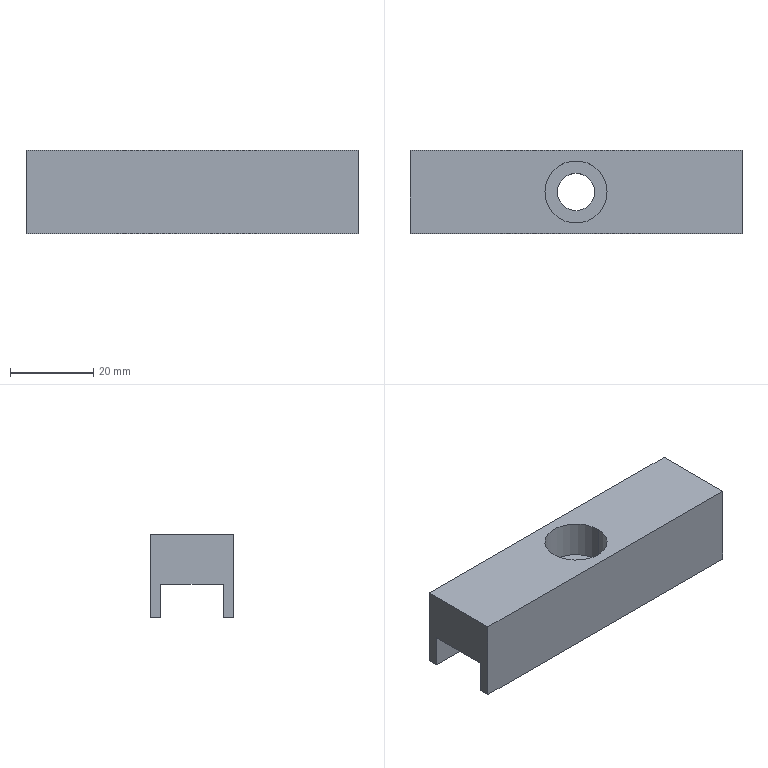Part | STEP file | Top plate part | 1 solid | 15 faces | box 80 x 20 x 20 mm | volume 20619 mm3 | plane 11 | cylinder 4 | commonest cylinder face diameters 9 x2 15 x2
STEP:
#1=CARTESIAN_POINT('',(0.,0.,0.));
#2=DIRECTION('',(0.,0.,1.));
#3=DIRECTION('',(1.,0.,0.));
#4=AXIS2_PLACEMENT_3D('',#1,#2,#3);
#5=CARTESIAN_POINT('',(7.5,0.,11.));
#6=VERTEX_POINT('',#5);
#7=CARTESIAN_POINT('',(7.5,0.,20.));
#8=VERTEX_POINT('',#7);
#9=CARTESIAN_POINT('',(7.5,0.,20.));
#10=DIRECTION('',(0.,0.,1.));
#11=VECTOR('',#10,1.);
#12=LINE('',#9,#11);
#13=CARTESIAN_POINT('',(0.,0.,20.));
#14=DIRECTION('',(0.,0.,1.));
#15=DIRECTION('',(1.,0.,0.));
#16=AXIS2_PLACEMENT_3D('',#13,#14,#15);
#17=CYLINDRICAL_SURFACE('',#16,7.5);
#18=CARTESIAN_POINT('',(6.283,0.));
#19=DIRECTION('',(0.,1.));
#20=VECTOR('',#19,1.);
#21=LINE('',#18,#20);
#22=(GEOMETRIC_REPRESENTATION_CONTEXT(2)PARAMETRIC_REPRESENTATION_CONTEXT()REPRESENTATION_CONTEXT('',''));
#23=DEFINITIONAL_REPRESENTATION('',(#21),#22);
#24=PCURVE('',#17,#23);
#25=CARTESIAN_POINT('',(0.,0.,20.));
#26=DIRECTION('',(0.,0.,1.));
#27=DIRECTION('',(1.,0.,0.));
#28=AXIS2_PLACEMENT_3D('',#25,#26,#27);
#29=CYLINDRICAL_SURFACE('',#28,7.5);
#30=CARTESIAN_POINT('',(0.,0.));
#31=DIRECTION('',(0.,1.));
#32=VECTOR('',#31,1.);
#33=LINE('',#30,#32);
#34=(GEOMETRIC_REPRESENTATION_CONTEXT(2)PARAMETRIC_REPRESENTATION_CONTEXT()REPRESENTATION_CONTEXT('',''));
#35=DEFINITIONAL_REPRESENTATION('',(#33),#34);
#36=PCURVE('',#29,#35);
#37=SURFACE_CURVE('',#12,(#24,#36),.PCURVE_S1.);
#38=EDGE_CURVE('',#6,#8,#37,.T.);
#39=ORIENTED_EDGE('',*,*,#38,.T.);
#40=CARTESIAN_POINT('',(-7.5,0.,20.));
#41=VERTEX_POINT('',#40);
#42=CARTESIAN_POINT('',(0.,0.,20.));
#43=DIRECTION('',(0.,0.,1.));
#44=DIRECTION('',(1.,0.,0.));
#45=AXIS2_PLACEMENT_3D('',#42,#43,#44);
#46=CIRCLE('',#45,7.5);
#47=CARTESIAN_POINT('',(0.,0.));
#48=DIRECTION('',(1.,0.));
#49=VECTOR('',#48,1.);
#50=LINE('',#47,#49);
#51=(GEOMETRIC_REPRESENTATION_CONTEXT(2)PARAMETRIC_REPRESENTATION_CONTEXT()REPRESENTATION_CONTEXT('',''));
#52=DEFINITIONAL_REPRESENTATION('',(#50),#51);
#53=PCURVE('',#17,#52);
#54=CARTESIAN_POINT('',(0.,0.,20.));
#55=DIRECTION('',(0.,0.,1.));
#56=DIRECTION('',(1.,0.,0.));
#57=AXIS2_PLACEMENT_3D('',#54,#55,#56);
#58=PLANE('',#57);
#59=CARTESIAN_POINT('',(0.,0.));
#60=DIRECTION('',(1.,0.));
#61=AXIS2_PLACEMENT_2D('',#59,#60);
#62=CIRCLE('',#61,7.5);
#63=(GEOMETRIC_REPRESENTATION_CONTEXT(2)PARAMETRIC_REPRESENTATION_CONTEXT()REPRESENTATION_CONTEXT('',''));
#64=DEFINITIONAL_REPRESENTATION('',(#62),#63);
#65=PCURVE('',#58,#64);
#66=SURFACE_CURVE('',#46,(#53,#65),.PCURVE_S1.);
#67=EDGE_CURVE('',#41,#8,#66,.T.);
#68=ORIENTED_EDGE('',*,*,#67,.F.);
#69=CARTESIAN_POINT('',(-7.5,0.,11.));
#70=VERTEX_POINT('',#69);
#71=CARTESIAN_POINT('',(-7.5,0.,20.));
#72=DIRECTION('',(0.,0.,1.));
#73=VECTOR('',#72,1.);
#74=LINE('',#71,#73);
#75=CARTESIAN_POINT('',(3.142,0.));
#76=DIRECTION('',(0.,1.));
#77=VECTOR('',#76,1.);
#78=LINE('',#75,#77);
#79=(GEOMETRIC_REPRESENTATION_CONTEXT(2)PARAMETRIC_REPRESENTATION_CONTEXT()REPRESENTATION_CONTEXT('',''));
#80=DEFINITIONAL_REPRESENTATION('',(#78),#79);
#81=PCURVE('',#17,#80);
#82=CARTESIAN_POINT('',(3.142,0.));
#83=DIRECTION('',(0.,1.));
#84=VECTOR('',#83,1.);
#85=LINE('',#82,#84);
#86=(GEOMETRIC_REPRESENTATION_CONTEXT(2)PARAMETRIC_REPRESENTATION_CONTEXT()REPRESENTATION_CONTEXT('',''));
#87=DEFINITIONAL_REPRESENTATION('',(#85),#86);
#88=PCURVE('',#29,#87);
#89=SURFACE_CURVE('',#74,(#81,#88),.PCURVE_S1.);
#90=EDGE_CURVE('',#70,#41,#89,.T.);
#91=ORIENTED_EDGE('',*,*,#90,.F.);
#92=CARTESIAN_POINT('',(0.,0.,11.));
#93=DIRECTION('',(0.,0.,1.));
#94=DIRECTION('',(1.,0.,0.));
#95=AXIS2_PLACEMENT_3D('',#92,#93,#94);
#96=CIRCLE('',#95,7.5);
#97=CARTESIAN_POINT('',(0.,-9.));
#98=DIRECTION('',(1.,0.));
#99=VECTOR('',#98,1.);
#100=LINE('',#97,#99);
#101=(GEOMETRIC_REPRESENTATION_CONTEXT(2)PARAMETRIC_REPRESENTATION_CONTEXT()REPRESENTATION_CONTEXT('',''));
#102=DEFINITIONAL_REPRESENTATION('',(#100),#101);
#103=PCURVE('',#17,#102);
#104=CARTESIAN_POINT('',(4.5,0.,11.));
#105=DIRECTION('',(0.,0.,-1.));
#106=DIRECTION('',(-1.,0.,0.));
#107=AXIS2_PLACEMENT_3D('',#104,#105,#106);
#108=PLANE('',#107);
#109=CARTESIAN_POINT('',(-3.,0.));
#110=CARTESIAN_POINT('',(-3.,12.99));
#111=CARTESIAN_POINT('',(8.25,6.495));
#112=CARTESIAN_POINT('',(19.5,0.));
#113=CARTESIAN_POINT('',(8.25,-6.495));
#114=CARTESIAN_POINT('',(-3.,-12.99));
#115=CARTESIAN_POINT('',(-3.,0.));
#116=(BOUNDED_CURVE()B_SPLINE_CURVE(2,(#109,#110,#111,#112,#113,#114,#115),.UNSPECIFIED.,.T.,.F.)B_SPLINE_CURVE_WITH_KNOTS((1,2,2,2,2,1),(-2.094,0.,2.094,4.189,6.283,8.378),.UNSPECIFIED.)CURVE()GEOMETRIC_REPRESENTATION_ITEM()RATIONAL_B_SPLINE_CURVE((1.,0.5,1.,0.5,1.,0.5,1.))REPRESENTATION_ITEM(''));
#117=(GEOMETRIC_REPRESENTATION_CONTEXT(2)PARAMETRIC_REPRESENTATION_CONTEXT()REPRESENTATION_CONTEXT('',''));
#118=DEFINITIONAL_REPRESENTATION('',(#116),#117);
#119=PCURVE('',#108,#118);
#120=SURFACE_CURVE('',#96,(#103,#119),.PCURVE_S1.);
#121=EDGE_CURVE('',#70,#6,#120,.T.);
#122=ORIENTED_EDGE('',*,*,#121,.T.);
#123=EDGE_LOOP('',(#39,#68,#91,#122));
#124=FACE_BOUND('',#123,.F.);
#125=ADVANCED_FACE('',(#124),#17,.F.);
#126=CARTESIAN_POINT('',(4.5,0.,8.));
#127=VERTEX_POINT('',#126);
#128=CARTESIAN_POINT('',(4.5,0.,11.));
#129=VERTEX_POINT('',#128);
#130=CARTESIAN_POINT('',(4.5,0.,20.));
#131=DIRECTION('',(0.,0.,1.));
#132=VECTOR('',#131,1.);
#133=LINE('',#130,#132);
#134=CARTESIAN_POINT('',(0.,0.,20.));
#135=DIRECTION('',(0.,0.,1.));
#136=DIRECTION('',(1.,0.,0.));
#137=AXIS2_PLACEMENT_3D('',#134,#135,#136);
#138=CYLINDRICAL_SURFACE('',#137,4.5);
#139=CARTESIAN_POINT('',(6.283,0.));
#140=DIRECTION('',(0.,1.));
#141=VECTOR('',#140,1.);
#142=LINE('',#139,#141);
#143=(GEOMETRIC_REPRESENTATION_CONTEXT(2)PARAMETRIC_REPRESENTATION_CONTEXT()REPRESENTATION_CONTEXT('',''));
#144=DEFINITIONAL_REPRESENTATION('',(#142),#143);
#145=PCURVE('',#138,#144);
#146=CARTESIAN_POINT('',(0.,0.,20.));
#147=DIRECTION('',(0.,0.,1.));
#148=DIRECTION('',(1.,0.,0.));
#149=AXIS2_PLACEMENT_3D('',#146,#147,#148);
#150=CYLINDRICAL_SURFACE('',#149,4.5);
#151=CARTESIAN_POINT('',(0.,0.));
#152=DIRECTION('',(0.,1.));
#153=VECTOR('',#152,1.);
#154=LINE('',#151,#153);
#155=(GEOMETRIC_REPRESENTATION_CONTEXT(2)PARAMETRIC_REPRESENTATION_CONTEXT()REPRESENTATION_CONTEXT('',''));
#156=DEFINITIONAL_REPRESENTATION('',(#154),#155);
#157=PCURVE('',#150,#156);
#158=SURFACE_CURVE('',#133,(#145,#157),.PCURVE_S1.);
#159=EDGE_CURVE('',#127,#129,#158,.T.);
#160=ORIENTED_EDGE('',*,*,#159,.T.);
#161=CARTESIAN_POINT('',(-4.5,0.,11.));
#162=VERTEX_POINT('',#161);
#163=CARTESIAN_POINT('',(0.,0.,11.));
#164=DIRECTION('',(0.,0.,1.));
#165=DIRECTION('',(1.,0.,0.));
#166=AXIS2_PLACEMENT_3D('',#163,#164,#165);
#167=CIRCLE('',#166,4.5);
#168=CARTESIAN_POINT('',(0.,-9.));
#169=DIRECTION('',(1.,0.));
#170=VECTOR('',#169,1.);
#171=LINE('',#168,#170);
#172=(GEOMETRIC_REPRESENTATION_CONTEXT(2)PARAMETRIC_REPRESENTATION_CONTEXT()REPRESENTATION_CONTEXT('',''));
#173=DEFINITIONAL_REPRESENTATION('',(#171),#172);
#174=PCURVE('',#138,#173);
#175=CARTESIAN_POINT('',(0.,0.));
#176=CARTESIAN_POINT('',(0.,7.794));
#177=CARTESIAN_POINT('',(6.75,3.897));
#178=CARTESIAN_POINT('',(13.5,0.));
#179=CARTESIAN_POINT('',(6.75,-3.897));
#180=CARTESIAN_POINT('',(0.,-7.794));
#181=CARTESIAN_POINT('',(0.,0.));
#182=(BOUNDED_CURVE()B_SPLINE_CURVE(2,(#175,#176,#177,#178,#179,#180,#181),.UNSPECIFIED.,.T.,.F.)B_SPLINE_CURVE_WITH_KNOTS((1,2,2,2,2,1),(-2.094,0.,2.094,4.189,6.283,8.378),.UNSPECIFIED.)CURVE()GEOMETRIC_REPRESENTATION_ITEM()RATIONAL_B_SPLINE_CURVE((1.,0.5,1.,0.5,1.,0.5,1.))REPRESENTATION_ITEM(''));
#183=(GEOMETRIC_REPRESENTATION_CONTEXT(2)PARAMETRIC_REPRESENTATION_CONTEXT()REPRESENTATION_CONTEXT('',''));
#184=DEFINITIONAL_REPRESENTATION('',(#182),#183);
#185=PCURVE('',#108,#184);
#186=SURFACE_CURVE('',#167,(#174,#185),.PCURVE_S1.);
#187=EDGE_CURVE('',#162,#129,#186,.T.);
#188=ORIENTED_EDGE('',*,*,#187,.F.);
#189=CARTESIAN_POINT('',(-4.5,0.,8.));
#190=VERTEX_POINT('',#189);
#191=CARTESIAN_POINT('',(-4.5,0.,20.));
#192=DIRECTION('',(0.,0.,1.));
#193=VECTOR('',#192,1.);
#194=LINE('',#191,#193);
#195=CARTESIAN_POINT('',(3.142,0.));
#196=DIRECTION('',(0.,1.));
#197=VECTOR('',#196,1.);
#198=LINE('',#195,#197);
#199=(GEOMETRIC_REPRESENTATION_CONTEXT(2)PARAMETRIC_REPRESENTATION_CONTEXT()REPRESENTATION_CONTEXT('',''));
#200=DEFINITIONAL_REPRESENTATION('',(#198),#199);
#201=PCURVE('',#138,#200);
#202=CARTESIAN_POINT('',(3.142,0.));
#203=DIRECTION('',(0.,1.));
#204=VECTOR('',#203,1.);
#205=LINE('',#202,#204);
#206=(GEOMETRIC_REPRESENTATION_CONTEXT(2)PARAMETRIC_REPRESENTATION_CONTEXT()REPRESENTATION_CONTEXT('',''));
#207=DEFINITIONAL_REPRESENTATION('',(#205),#206);
#208=PCURVE('',#150,#207);
#209=SURFACE_CURVE('',#194,(#201,#208),.PCURVE_S1.);
#210=EDGE_CURVE('',#190,#162,#209,.T.);
#211=ORIENTED_EDGE('',*,*,#210,.F.);
#212=CARTESIAN_POINT('',(0.,0.,8.));
#213=DIRECTION('',(0.,0.,1.));
#214=DIRECTION('',(1.,0.,0.));
#215=AXIS2_PLACEMENT_3D('',#212,#213,#214);
#216=CIRCLE('',#215,4.5);
#217=CARTESIAN_POINT('',(0.,-12.));
#218=DIRECTION('',(1.,0.));
#219=VECTOR('',#218,1.);
#220=LINE('',#217,#219);
#221=(GEOMETRIC_REPRESENTATION_CONTEXT(2)PARAMETRIC_REPRESENTATION_CONTEXT()REPRESENTATION_CONTEXT('',''));
#222=DEFINITIONAL_REPRESENTATION('',(#220),#221);
#223=PCURVE('',#138,#222);
#224=CARTESIAN_POINT('',(-40.,7.5,8.));
#225=DIRECTION('',(0.,0.,1.));
#226=DIRECTION('',(1.,0.,0.));
#227=AXIS2_PLACEMENT_3D('',#224,#225,#226);
#228=PLANE('',#227);
#229=CARTESIAN_POINT('',(40.,-7.5));
#230=DIRECTION('',(1.,0.));
#231=AXIS2_PLACEMENT_2D('',#229,#230);
#232=CIRCLE('',#231,4.5);
#233=(GEOMETRIC_REPRESENTATION_CONTEXT(2)PARAMETRIC_REPRESENTATION_CONTEXT()REPRESENTATION_CONTEXT('',''));
#234=DEFINITIONAL_REPRESENTATION('',(#232),#233);
#235=PCURVE('',#228,#234);
#236=SURFACE_CURVE('',#216,(#223,#235),.PCURVE_S1.);
#237=EDGE_CURVE('',#190,#127,#236,.T.);
#238=ORIENTED_EDGE('',*,*,#237,.T.);
#239=EDGE_LOOP('',(#160,#188,#211,#238));
#240=FACE_BOUND('',#239,.F.);
#241=ADVANCED_FACE('',(#240),#138,.F.);
#242=CARTESIAN_POINT('',(40.,7.5,0.));
#243=VERTEX_POINT('',#242);
#244=CARTESIAN_POINT('',(40.,10.,0.));
#245=VERTEX_POINT('',#244);
#246=CARTESIAN_POINT('',(40.,10.,0.));
#247=DIRECTION('',(0.,1.,0.));
#248=VECTOR('',#247,1.);
#249=LINE('',#246,#248);
#250=CARTESIAN_POINT('',(0.,0.,0.));
#251=DIRECTION('',(0.,0.,1.));
#252=DIRECTION('',(1.,0.,0.));
#253=AXIS2_PLACEMENT_3D('',#250,#251,#252);
#254=PLANE('',#253);
#255=CARTESIAN_POINT('',(40.,10.));
#256=DIRECTION('',(0.,1.));
#257=VECTOR('',#256,1.);
#258=LINE('',#255,#257);
#259=(GEOMETRIC_REPRESENTATION_CONTEXT(2)PARAMETRIC_REPRESENTATION_CONTEXT()REPRESENTATION_CONTEXT('',''));
#260=DEFINITIONAL_REPRESENTATION('',(#258),#259);
#261=PCURVE('',#254,#260);
#262=CARTESIAN_POINT('',(40.,10.,20.));
#263=DIRECTION('',(-1.,0.,0.));
#264=DIRECTION('',(0.,-1.,0.));
#265=AXIS2_PLACEMENT_3D('',#262,#263,#264);
#266=PLANE('',#265);
#267=CARTESIAN_POINT('',(0.,-20.));
#268=DIRECTION('',(-1.,0.));
#269=VECTOR('',#268,1.);
#270=LINE('',#267,#269);
#271=(GEOMETRIC_REPRESENTATION_CONTEXT(2)PARAMETRIC_REPRESENTATION_CONTEXT()REPRESENTATION_CONTEXT('',''));
#272=DEFINITIONAL_REPRESENTATION('',(#270),#271);
#273=PCURVE('',#266,#272);
#274=SURFACE_CURVE('',#249,(#261,#273),.PCURVE_S1.);
#275=EDGE_CURVE('',#243,#245,#274,.T.);
#276=ORIENTED_EDGE('',*,*,#275,.F.);
#277=CARTESIAN_POINT('',(-40.,7.5,0.));
#278=VERTEX_POINT('',#277);
#279=CARTESIAN_POINT('',(0.,7.5,0.));
#280=DIRECTION('',(-1.,0.,0.));
#281=VECTOR('',#280,1.);
#282=LINE('',#279,#281);
#283=CARTESIAN_POINT('',(0.,7.5));
#284=DIRECTION('',(-1.,0.));
#285=VECTOR('',#284,1.);
#286=LINE('',#283,#285);
#287=(GEOMETRIC_REPRESENTATION_CONTEXT(2)PARAMETRIC_REPRESENTATION_CONTEXT()REPRESENTATION_CONTEXT('',''));
#288=DEFINITIONAL_REPRESENTATION('',(#286),#287);
#289=PCURVE('',#254,#288);
#290=CARTESIAN_POINT('',(-40.,7.5,-8.));
#291=DIRECTION('',(0.,1.,0.));
#292=DIRECTION('',(0.,0.,1.));
#293=AXIS2_PLACEMENT_3D('',#290,#291,#292);
#294=PLANE('',#293);
#295=CARTESIAN_POINT('',(8.,40.));
#296=DIRECTION('',(0.,-1.));
#297=VECTOR('',#296,1.);
#298=LINE('',#295,#297);
#299=(GEOMETRIC_REPRESENTATION_CONTEXT(2)PARAMETRIC_REPRESENTATION_CONTEXT()REPRESENTATION_CONTEXT('',''));
#300=DEFINITIONAL_REPRESENTATION('',(#298),#299);
#301=PCURVE('',#294,#300);
#302=SURFACE_CURVE('',#282,(#289,#301),.PCURVE_S1.);
#303=EDGE_CURVE('',#243,#278,#302,.T.);
#304=ORIENTED_EDGE('',*,*,#303,.T.);
#305=CARTESIAN_POINT('',(-40.,10.,0.));
#306=VERTEX_POINT('',#305);
#307=CARTESIAN_POINT('',(-40.,10.,0.));
#308=DIRECTION('',(0.,-1.,0.));
#309=VECTOR('',#308,1.);
#310=LINE('',#307,#309);
#311=CARTESIAN_POINT('',(-40.,10.));
#312=DIRECTION('',(0.,-1.));
#313=VECTOR('',#312,1.);
#314=LINE('',#311,#313);
#315=(GEOMETRIC_REPRESENTATION_CONTEXT(2)PARAMETRIC_REPRESENTATION_CONTEXT()REPRESENTATION_CONTEXT('',''));
#316=DEFINITIONAL_REPRESENTATION('',(#314),#315);
#317=PCURVE('',#254,#316);
#318=CARTESIAN_POINT('',(-40.,10.,20.));
#319=DIRECTION('',(1.,0.,0.));
#320=DIRECTION('',(0.,0.,-1.));
#321=AXIS2_PLACEMENT_3D('',#318,#319,#320);
#322=PLANE('',#321);
#323=CARTESIAN_POINT('',(20.,0.));
#324=DIRECTION('',(0.,-1.));
#325=VECTOR('',#324,1.);
#326=LINE('',#323,#325);
#327=(GEOMETRIC_REPRESENTATION_CONTEXT(2)PARAMETRIC_REPRESENTATION_CONTEXT()REPRESENTATION_CONTEXT('',''));
#328=DEFINITIONAL_REPRESENTATION('',(#326),#327);
#329=PCURVE('',#322,#328);
#330=SURFACE_CURVE('',#310,(#317,#329),.PCURVE_S1.);
#331=EDGE_CURVE('',#306,#278,#330,.T.);
#332=ORIENTED_EDGE('',*,*,#331,.F.);
#333=CARTESIAN_POINT('',(-40.,10.,0.));
#334=DIRECTION('',(-1.,0.,0.));
#335=VECTOR('',#334,1.);
#336=LINE('',#333,#335);
#337=CARTESIAN_POINT('',(-40.,10.));
#338=DIRECTION('',(-1.,0.));
#339=VECTOR('',#338,1.);
#340=LINE('',#337,#339);
#341=(GEOMETRIC_REPRESENTATION_CONTEXT(2)PARAMETRIC_REPRESENTATION_CONTEXT()REPRESENTATION_CONTEXT('',''));
#342=DEFINITIONAL_REPRESENTATION('',(#340),#341);
#343=PCURVE('',#254,#342);
#344=CARTESIAN_POINT('',(-40.,10.,20.));
#345=DIRECTION('',(0.,-1.,0.));
#346=DIRECTION('',(0.,0.,-1.));
#347=AXIS2_PLACEMENT_3D('',#344,#345,#346);
#348=PLANE('',#347);
#349=CARTESIAN_POINT('',(20.,0.));
#350=DIRECTION('',(0.,-1.));
#351=VECTOR('',#350,1.);
#352=LINE('',#349,#351);
#353=(GEOMETRIC_REPRESENTATION_CONTEXT(2)PARAMETRIC_REPRESENTATION_CONTEXT()REPRESENTATION_CONTEXT('',''));
#354=DEFINITIONAL_REPRESENTATION('',(#352),#353);
#355=PCURVE('',#348,#354);
#356=SURFACE_CURVE('',#336,(#343,#355),.PCURVE_S1.);
#357=EDGE_CURVE('',#245,#306,#356,.T.);
#358=ORIENTED_EDGE('',*,*,#357,.F.);
#359=EDGE_LOOP('',(#276,#304,#332,#358));
#360=FACE_BOUND('',#359,.T.);
#361=ADVANCED_FACE('',(#360),#254,.F.);
#362=CARTESIAN_POINT('',(40.,7.5,8.));
#363=VERTEX_POINT('',#362);
#364=CARTESIAN_POINT('',(40.,-7.5,8.));
#365=VERTEX_POINT('',#364);
#366=CARTESIAN_POINT('',(40.,7.5,8.));
#367=DIRECTION('',(0.,-1.,0.));
#368=VECTOR('',#367,1.);
#369=LINE('',#366,#368);
#370=CARTESIAN_POINT('',(2.5,-12.));
#371=DIRECTION('',(1.,0.));
#372=VECTOR('',#371,1.);
#373=LINE('',#370,#372);
#374=(GEOMETRIC_REPRESENTATION_CONTEXT(2)PARAMETRIC_REPRESENTATION_CONTEXT()REPRESENTATION_CONTEXT('',''));
#375=DEFINITIONAL_REPRESENTATION('',(#373),#374);
#376=PCURVE('',#266,#375);
#377=CARTESIAN_POINT('',(80.,0.));
#378=DIRECTION('',(0.,-1.));
#379=VECTOR('',#378,1.);
#380=LINE('',#377,#379);
#381=(GEOMETRIC_REPRESENTATION_CONTEXT(2)PARAMETRIC_REPRESENTATION_CONTEXT()REPRESENTATION_CONTEXT('',''));
#382=DEFINITIONAL_REPRESENTATION('',(#380),#381);
#383=PCURVE('',#228,#382);
#384=SURFACE_CURVE('',#369,(#376,#383),.PCURVE_S1.);
#385=EDGE_CURVE('',#363,#365,#384,.T.);
#386=ORIENTED_EDGE('',*,*,#385,.F.);
#387=CARTESIAN_POINT('',(40.,7.5,-8.));
#388=DIRECTION('',(0.,0.,1.));
#389=VECTOR('',#388,1.);
#390=LINE('',#387,#389);
#391=CARTESIAN_POINT('',(2.5,-28.));
#392=DIRECTION('',(0.,1.));
#393=VECTOR('',#392,1.);
#394=LINE('',#391,#393);
#395=(GEOMETRIC_REPRESENTATION_CONTEXT(2)PARAMETRIC_REPRESENTATION_CONTEXT()REPRESENTATION_CONTEXT('',''));
#396=DEFINITIONAL_REPRESENTATION('',(#394),#395);
#397=PCURVE('',#266,#396);
#398=CARTESIAN_POINT('',(0.,80.));
#399=DIRECTION('',(1.,0.));
#400=VECTOR('',#399,1.);
#401=LINE('',#398,#400);
#402=(GEOMETRIC_REPRESENTATION_CONTEXT(2)PARAMETRIC_REPRESENTATION_CONTEXT()REPRESENTATION_CONTEXT('',''));
#403=DEFINITIONAL_REPRESENTATION('',(#401),#402);
#404=PCURVE('',#294,#403);
#405=SURFACE_CURVE('',#390,(#397,#404),.PCURVE_S1.);
#406=EDGE_CURVE('',#243,#363,#405,.T.);
#407=ORIENTED_EDGE('',*,*,#406,.F.);
#408=ORIENTED_EDGE('',*,*,#275,.T.);
#409=CARTESIAN_POINT('',(40.,10.,20.));
#410=VERTEX_POINT('',#409);
#411=CARTESIAN_POINT('',(40.,10.,20.));
#412=DIRECTION('',(0.,0.,-1.));
#413=VECTOR('',#412,1.);
#414=LINE('',#411,#413);
#415=CARTESIAN_POINT('',(0.,0.));
#416=DIRECTION('',(0.,-1.));
#417=VECTOR('',#416,1.);
#418=LINE('',#415,#417);
#419=(GEOMETRIC_REPRESENTATION_CONTEXT(2)PARAMETRIC_REPRESENTATION_CONTEXT()REPRESENTATION_CONTEXT('',''));
#420=DEFINITIONAL_REPRESENTATION('',(#418),#419);
#421=PCURVE('',#266,#420);
#422=CARTESIAN_POINT('',(0.,80.));
#423=DIRECTION('',(1.,0.));
#424=VECTOR('',#423,1.);
#425=LINE('',#422,#424);
#426=(GEOMETRIC_REPRESENTATION_CONTEXT(2)PARAMETRIC_REPRESENTATION_CONTEXT()REPRESENTATION_CONTEXT('',''));
#427=DEFINITIONAL_REPRESENTATION('',(#425),#426);
#428=PCURVE('',#348,#427);
#429=SURFACE_CURVE('',#414,(#421,#428),.PCURVE_S1.);
#430=EDGE_CURVE('',#410,#245,#429,.T.);
#431=ORIENTED_EDGE('',*,*,#430,.F.);
#432=CARTESIAN_POINT('',(40.,-10.,20.));
#433=VERTEX_POINT('',#432);
#434=CARTESIAN_POINT('',(40.,10.,20.));
#435=DIRECTION('',(0.,1.,0.));
#436=VECTOR('',#435,1.);
#437=LINE('',#434,#436);
#438=CARTESIAN_POINT('',(0.,0.));
#439=DIRECTION('',(-1.,0.));
#440=VECTOR('',#439,1.);
#441=LINE('',#438,#440);
#442=(GEOMETRIC_REPRESENTATION_CONTEXT(2)PARAMETRIC_REPRESENTATION_CONTEXT()REPRESENTATION_CONTEXT('',''));
#443=DEFINITIONAL_REPRESENTATION('',(#441),#442);
#444=PCURVE('',#266,#443);
#445=CARTESIAN_POINT('',(40.,10.));
#446=DIRECTION('',(0.,1.));
#447=VECTOR('',#446,1.);
#448=LINE('',#445,#447);
#449=(GEOMETRIC_REPRESENTATION_CONTEXT(2)PARAMETRIC_REPRESENTATION_CONTEXT()REPRESENTATION_CONTEXT('',''));
#450=DEFINITIONAL_REPRESENTATION('',(#448),#449);
#451=PCURVE('',#58,#450);
#452=SURFACE_CURVE('',#437,(#444,#451),.PCURVE_S1.);
#453=EDGE_CURVE('',#433,#410,#452,.T.);
#454=ORIENTED_EDGE('',*,*,#453,.F.);
#455=CARTESIAN_POINT('',(40.,-10.,0.));
#456=VERTEX_POINT('',#455);
#457=CARTESIAN_POINT('',(40.,-10.,20.));
#458=DIRECTION('',(0.,0.,-1.));
#459=VECTOR('',#458,1.);
#460=LINE('',#457,#459);
#461=CARTESIAN_POINT('',(20.,0.));
#462=DIRECTION('',(0.,-1.));
#463=VECTOR('',#462,1.);
#464=LINE('',#461,#463);
#465=(GEOMETRIC_REPRESENTATION_CONTEXT(2)PARAMETRIC_REPRESENTATION_CONTEXT()REPRESENTATION_CONTEXT('',''));
#466=DEFINITIONAL_REPRESENTATION('',(#464),#465);
#467=PCURVE('',#266,#466);
#468=CARTESIAN_POINT('',(-40.,-10.,20.));
#469=DIRECTION('',(0.,1.,0.));
#470=DIRECTION('',(0.,0.,1.));
#471=AXIS2_PLACEMENT_3D('',#468,#469,#470);
#472=PLANE('',#471);
#473=CARTESIAN_POINT('',(0.,80.));
#474=DIRECTION('',(-1.,0.));
#475=VECTOR('',#474,1.);
#476=LINE('',#473,#475);
#477=(GEOMETRIC_REPRESENTATION_CONTEXT(2)PARAMETRIC_REPRESENTATION_CONTEXT()REPRESENTATION_CONTEXT('',''));
#478=DEFINITIONAL_REPRESENTATION('',(#476),#477);
#479=PCURVE('',#472,#478);
#480=SURFACE_CURVE('',#460,(#467,#479),.PCURVE_S1.);
#481=EDGE_CURVE('',#433,#456,#480,.T.);
#482=ORIENTED_EDGE('',*,*,#481,.T.);
#483=CARTESIAN_POINT('',(40.,-7.5,0.));
#484=VERTEX_POINT('',#483);
#485=CARTESIAN_POINT('',(40.,10.,0.));
#486=DIRECTION('',(0.,1.,0.));
#487=VECTOR('',#486,1.);
#488=LINE('',#485,#487);
#489=CARTESIAN_POINT('',(0.,-20.));
#490=DIRECTION('',(-1.,0.));
#491=VECTOR('',#490,1.);
#492=LINE('',#489,#491);
#493=(GEOMETRIC_REPRESENTATION_CONTEXT(2)PARAMETRIC_REPRESENTATION_CONTEXT()REPRESENTATION_CONTEXT('',''));
#494=DEFINITIONAL_REPRESENTATION('',(#492),#493);
#495=PCURVE('',#266,#494);
#496=CARTESIAN_POINT('',(0.,0.,0.));
#497=DIRECTION('',(0.,0.,1.));
#498=DIRECTION('',(1.,0.,0.));
#499=AXIS2_PLACEMENT_3D('',#496,#497,#498);
#500=PLANE('',#499);
#501=CARTESIAN_POINT('',(40.,10.));
#502=DIRECTION('',(0.,1.));
#503=VECTOR('',#502,1.);
#504=LINE('',#501,#503);
#505=(GEOMETRIC_REPRESENTATION_CONTEXT(2)PARAMETRIC_REPRESENTATION_CONTEXT()REPRESENTATION_CONTEXT('',''));
#506=DEFINITIONAL_REPRESENTATION('',(#504),#505);
#507=PCURVE('',#500,#506);
#508=SURFACE_CURVE('',#488,(#495,#507),.PCURVE_S1.);
#509=EDGE_CURVE('',#456,#484,#508,.T.);
#510=ORIENTED_EDGE('',*,*,#509,.T.);
#511=CARTESIAN_POINT('',(40.,-7.5,-8.));
#512=DIRECTION('',(0.,0.,-1.));
#513=VECTOR('',#512,1.);
#514=LINE('',#511,#513);
#515=CARTESIAN_POINT('',(17.5,-28.));
#516=DIRECTION('',(0.,-1.));
#517=VECTOR('',#516,1.);
#518=LINE('',#515,#517);
#519=(GEOMETRIC_REPRESENTATION_CONTEXT(2)PARAMETRIC_REPRESENTATION_CONTEXT()REPRESENTATION_CONTEXT('',''));
#520=DEFINITIONAL_REPRESENTATION('',(#518),#519);
#521=PCURVE('',#266,#520);
#522=CARTESIAN_POINT('',(-40.,-7.5,-8.));
#523=DIRECTION('',(0.,-1.,0.));
#524=DIRECTION('',(0.,0.,-1.));
#525=AXIS2_PLACEMENT_3D('',#522,#523,#524);
#526=PLANE('',#525);
#527=CARTESIAN_POINT('',(0.,80.));
#528=DIRECTION('',(1.,0.));
#529=VECTOR('',#528,1.);
#530=LINE('',#527,#529);
#531=(GEOMETRIC_REPRESENTATION_CONTEXT(2)PARAMETRIC_REPRESENTATION_CONTEXT()REPRESENTATION_CONTEXT('',''));
#532=DEFINITIONAL_REPRESENTATION('',(#530),#531);
#533=PCURVE('',#526,#532);
#534=SURFACE_CURVE('',#514,(#521,#533),.PCURVE_S1.);
#535=EDGE_CURVE('',#365,#484,#534,.T.);
#536=ORIENTED_EDGE('',*,*,#535,.F.);
#537=EDGE_LOOP('',(#386,#407,#408,#431,#454,#482,#510,#536));
#538=FACE_BOUND('',#537,.T.);
#539=ADVANCED_FACE('',(#538),#266,.F.);
#540=ORIENTED_EDGE('',*,*,#357,.T.);
#541=CARTESIAN_POINT('',(-40.,10.,20.));
#542=VERTEX_POINT('',#541);
#543=CARTESIAN_POINT('',(-40.,10.,20.));
#544=DIRECTION('',(0.,0.,-1.));
#545=VECTOR('',#544,1.);
#546=LINE('',#543,#545);
#547=CARTESIAN_POINT('',(0.,0.));
#548=DIRECTION('',(1.,0.));
#549=VECTOR('',#548,1.);
#550=LINE('',#547,#549);
#551=(GEOMETRIC_REPRESENTATION_CONTEXT(2)PARAMETRIC_REPRESENTATION_CONTEXT()REPRESENTATION_CONTEXT('',''));
#552=DEFINITIONAL_REPRESENTATION('',(#550),#551);
#553=PCURVE('',#348,#552);
#554=CARTESIAN_POINT('',(0.,0.));
#555=DIRECTION('',(1.,0.));
#556=VECTOR('',#555,1.);
#557=LINE('',#554,#556);
#558=(GEOMETRIC_REPRESENTATION_CONTEXT(2)PARAMETRIC_REPRESENTATION_CONTEXT()REPRESENTATION_CONTEXT('',''));
#559=DEFINITIONAL_REPRESENTATION('',(#557),#558);
#560=PCURVE('',#322,#559);
#561=SURFACE_CURVE('',#546,(#553,#560),.PCURVE_S1.);
#562=EDGE_CURVE('',#542,#306,#561,.T.);
#563=ORIENTED_EDGE('',*,*,#562,.F.);
#564=CARTESIAN_POINT('',(-40.,10.,20.));
#565=DIRECTION('',(-1.,0.,0.));
#566=VECTOR('',#565,1.);
#567=LINE('',#564,#566);
#568=CARTESIAN_POINT('',(0.,0.));
#569=DIRECTION('',(0.,-1.));
#570=VECTOR('',#569,1.);
#571=LINE('',#568,#570);
#572=(GEOMETRIC_REPRESENTATION_CONTEXT(2)PARAMETRIC_REPRESENTATION_CONTEXT()REPRESENTATION_CONTEXT('',''));
#573=DEFINITIONAL_REPRESENTATION('',(#571),#572);
#574=PCURVE('',#348,#573);
#575=CARTESIAN_POINT('',(-40.,10.));
#576=DIRECTION('',(-1.,0.));
#577=VECTOR('',#576,1.);
#578=LINE('',#575,#577);
#579=(GEOMETRIC_REPRESENTATION_CONTEXT(2)PARAMETRIC_REPRESENTATION_CONTEXT()REPRESENTATION_CONTEXT('',''));
#580=DEFINITIONAL_REPRESENTATION('',(#578),#579);
#581=PCURVE('',#58,#580);
#582=SURFACE_CURVE('',#567,(#574,#581),.PCURVE_S1.);
#583=EDGE_CURVE('',#410,#542,#582,.T.);
#584=ORIENTED_EDGE('',*,*,#583,.F.);
#585=ORIENTED_EDGE('',*,*,#430,.T.);
#586=EDGE_LOOP('',(#540,#563,#584,#585));
#587=FACE_BOUND('',#586,.T.);
#588=ADVANCED_FACE('',(#587),#348,.F.);
#589=ORIENTED_EDGE('',*,*,#331,.T.);
#590=CARTESIAN_POINT('',(-40.,7.5,8.));
#591=VERTEX_POINT('',#590);
#592=CARTESIAN_POINT('',(-40.,7.5,-8.));
#593=DIRECTION('',(0.,0.,1.));
#594=VECTOR('',#593,1.);
#595=LINE('',#592,#594);
#596=CARTESIAN_POINT('',(28.,-2.5));
#597=DIRECTION('',(-1.,0.));
#598=VECTOR('',#597,1.);
#599=LINE('',#596,#598);
#600=(GEOMETRIC_REPRESENTATION_CONTEXT(2)PARAMETRIC_REPRESENTATION_CONTEXT()REPRESENTATION_CONTEXT('',''));
#601=DEFINITIONAL_REPRESENTATION('',(#599),#600);
#602=PCURVE('',#322,#601);
#603=CARTESIAN_POINT('',(0.,0.));
#604=DIRECTION('',(1.,0.));
#605=VECTOR('',#604,1.);
#606=LINE('',#603,#605);
#607=(GEOMETRIC_REPRESENTATION_CONTEXT(2)PARAMETRIC_REPRESENTATION_CONTEXT()REPRESENTATION_CONTEXT('',''));
#608=DEFINITIONAL_REPRESENTATION('',(#606),#607);
#609=PCURVE('',#294,#608);
#610=SURFACE_CURVE('',#595,(#602,#609),.PCURVE_S1.);
#611=EDGE_CURVE('',#278,#591,#610,.T.);
#612=ORIENTED_EDGE('',*,*,#611,.T.);
#613=CARTESIAN_POINT('',(-40.,-7.5,8.));
#614=VERTEX_POINT('',#613);
#615=CARTESIAN_POINT('',(-40.,7.5,8.));
#616=DIRECTION('',(0.,-1.,0.));
#617=VECTOR('',#616,1.);
#618=LINE('',#615,#617);
#619=CARTESIAN_POINT('',(12.,-2.5));
#620=DIRECTION('',(0.,-1.));
#621=VECTOR('',#620,1.);
#622=LINE('',#619,#621);
#623=(GEOMETRIC_REPRESENTATION_CONTEXT(2)PARAMETRIC_REPRESENTATION_CONTEXT()REPRESENTATION_CONTEXT('',''));
#624=DEFINITIONAL_REPRESENTATION('',(#622),#623);
#625=PCURVE('',#322,#624);
#626=CARTESIAN_POINT('',(0.,0.));
#627=DIRECTION('',(0.,-1.));
#628=VECTOR('',#627,1.);
#629=LINE('',#626,#628);
#630=(GEOMETRIC_REPRESENTATION_CONTEXT(2)PARAMETRIC_REPRESENTATION_CONTEXT()REPRESENTATION_CONTEXT('',''));
#631=DEFINITIONAL_REPRESENTATION('',(#629),#630);
#632=PCURVE('',#228,#631);
#633=SURFACE_CURVE('',#618,(#625,#632),.PCURVE_S1.);
#634=EDGE_CURVE('',#591,#614,#633,.T.);
#635=ORIENTED_EDGE('',*,*,#634,.T.);
#636=CARTESIAN_POINT('',(-40.,-7.5,0.));
#637=VERTEX_POINT('',#636);
#638=CARTESIAN_POINT('',(-40.,-7.5,-8.));
#639=DIRECTION('',(0.,0.,-1.));
#640=VECTOR('',#639,1.);
#641=LINE('',#638,#640);
#642=CARTESIAN_POINT('',(28.,-17.5));
#643=DIRECTION('',(1.,0.));
#644=VECTOR('',#643,1.);
#645=LINE('',#642,#644);
#646=(GEOMETRIC_REPRESENTATION_CONTEXT(2)PARAMETRIC_REPRESENTATION_CONTEXT()REPRESENTATION_CONTEXT('',''));
#647=DEFINITIONAL_REPRESENTATION('',(#645),#646);
#648=PCURVE('',#322,#647);
#649=CARTESIAN_POINT('',(0.,0.));
#650=DIRECTION('',(1.,0.));
#651=VECTOR('',#650,1.);
#652=LINE('',#649,#651);
#653=(GEOMETRIC_REPRESENTATION_CONTEXT(2)PARAMETRIC_REPRESENTATION_CONTEXT()REPRESENTATION_CONTEXT('',''));
#654=DEFINITIONAL_REPRESENTATION('',(#652),#653);
#655=PCURVE('',#526,#654);
#656=SURFACE_CURVE('',#641,(#648,#655),.PCURVE_S1.);
#657=EDGE_CURVE('',#614,#637,#656,.T.);
#658=ORIENTED_EDGE('',*,*,#657,.T.);
#659=CARTESIAN_POINT('',(-40.,-10.,0.));
#660=VERTEX_POINT('',#659);
#661=CARTESIAN_POINT('',(-40.,10.,0.));
#662=DIRECTION('',(0.,-1.,0.));
#663=VECTOR('',#662,1.);
#664=LINE('',#661,#663);
#665=CARTESIAN_POINT('',(20.,0.));
#666=DIRECTION('',(0.,-1.));
#667=VECTOR('',#666,1.);
#668=LINE('',#665,#667);
#669=(GEOMETRIC_REPRESENTATION_CONTEXT(2)PARAMETRIC_REPRESENTATION_CONTEXT()REPRESENTATION_CONTEXT('',''));
#670=DEFINITIONAL_REPRESENTATION('',(#668),#669);
#671=PCURVE('',#322,#670);
#672=CARTESIAN_POINT('',(-40.,10.));
#673=DIRECTION('',(0.,-1.));
#674=VECTOR('',#673,1.);
#675=LINE('',#672,#674);
#676=(GEOMETRIC_REPRESENTATION_CONTEXT(2)PARAMETRIC_REPRESENTATION_CONTEXT()REPRESENTATION_CONTEXT('',''));
#677=DEFINITIONAL_REPRESENTATION('',(#675),#676);
#678=PCURVE('',#500,#677);
#679=SURFACE_CURVE('',#664,(#671,#678),.PCURVE_S1.);
#680=EDGE_CURVE('',#637,#660,#679,.T.);
#681=ORIENTED_EDGE('',*,*,#680,.T.);
#682=CARTESIAN_POINT('',(-40.,-10.,20.));
#683=VERTEX_POINT('',#682);
#684=CARTESIAN_POINT('',(-40.,-10.,20.));
#685=DIRECTION('',(0.,0.,-1.));
#686=VECTOR('',#685,1.);
#687=LINE('',#684,#686);
#688=CARTESIAN_POINT('',(0.,-20.));
#689=DIRECTION('',(1.,0.));
#690=VECTOR('',#689,1.);
#691=LINE('',#688,#690);
#692=(GEOMETRIC_REPRESENTATION_CONTEXT(2)PARAMETRIC_REPRESENTATION_CONTEXT()REPRESENTATION_CONTEXT('',''));
#693=DEFINITIONAL_REPRESENTATION('',(#691),#692);
#694=PCURVE('',#322,#693);
#695=CARTESIAN_POINT('',(0.,0.));
#696=DIRECTION('',(-1.,0.));
#697=VECTOR('',#696,1.);
#698=LINE('',#695,#697);
#699=(GEOMETRIC_REPRESENTATION_CONTEXT(2)PARAMETRIC_REPRESENTATION_CONTEXT()REPRESENTATION_CONTEXT('',''));
#700=DEFINITIONAL_REPRESENTATION('',(#698),#699);
#701=PCURVE('',#472,#700);
#702=SURFACE_CURVE('',#687,(#694,#701),.PCURVE_S1.);
#703=EDGE_CURVE('',#683,#660,#702,.T.);
#704=ORIENTED_EDGE('',*,*,#703,.F.);
#705=CARTESIAN_POINT('',(-40.,10.,20.));
#706=DIRECTION('',(0.,-1.,0.));
#707=VECTOR('',#706,1.);
#708=LINE('',#705,#707);
#709=CARTESIAN_POINT('',(0.,0.));
#710=DIRECTION('',(0.,-1.));
#711=VECTOR('',#710,1.);
#712=LINE('',#709,#711);
#713=(GEOMETRIC_REPRESENTATION_CONTEXT(2)PARAMETRIC_REPRESENTATION_CONTEXT()REPRESENTATION_CONTEXT('',''));
#714=DEFINITIONAL_REPRESENTATION('',(#712),#713);
#715=PCURVE('',#322,#714);
#716=CARTESIAN_POINT('',(-40.,10.));
#717=DIRECTION('',(0.,-1.));
#718=VECTOR('',#717,1.);
#719=LINE('',#716,#718);
#720=(GEOMETRIC_REPRESENTATION_CONTEXT(2)PARAMETRIC_REPRESENTATION_CONTEXT()REPRESENTATION_CONTEXT('',''));
#721=DEFINITIONAL_REPRESENTATION('',(#719),#720);
#722=PCURVE('',#58,#721);
#723=SURFACE_CURVE('',#708,(#715,#722),.PCURVE_S1.);
#724=EDGE_CURVE('',#542,#683,#723,.T.);
#725=ORIENTED_EDGE('',*,*,#724,.F.);
#726=ORIENTED_EDGE('',*,*,#562,.T.);
#727=EDGE_LOOP('',(#589,#612,#635,#658,#681,#704,#725,#726));
#728=FACE_BOUND('',#727,.T.);
#729=ADVANCED_FACE('',(#728),#322,.F.);
#730=CARTESIAN_POINT('',(-40.,-10.,0.));
#731=DIRECTION('',(1.,0.,0.));
#732=VECTOR('',#731,1.);
#733=LINE('',#730,#732);
#734=CARTESIAN_POINT('',(-20.,0.));
#735=DIRECTION('',(0.,1.));
#736=VECTOR('',#735,1.);
#737=LINE('',#734,#736);
#738=(GEOMETRIC_REPRESENTATION_CONTEXT(2)PARAMETRIC_REPRESENTATION_CONTEXT()REPRESENTATION_CONTEXT('',''));
#739=DEFINITIONAL_REPRESENTATION('',(#737),#738);
#740=PCURVE('',#472,#739);
#741=CARTESIAN_POINT('',(-40.,-10.));
#742=DIRECTION('',(1.,0.));
#743=VECTOR('',#742,1.);
#744=LINE('',#741,#743);
#745=(GEOMETRIC_REPRESENTATION_CONTEXT(2)PARAMETRIC_REPRESENTATION_CONTEXT()REPRESENTATION_CONTEXT('',''));
#746=DEFINITIONAL_REPRESENTATION('',(#744),#745);
#747=PCURVE('',#500,#746);
#748=SURFACE_CURVE('',#733,(#740,#747),.PCURVE_S1.);
#749=EDGE_CURVE('',#660,#456,#748,.T.);
#750=ORIENTED_EDGE('',*,*,#749,.T.);
#751=ORIENTED_EDGE('',*,*,#481,.F.);
#752=CARTESIAN_POINT('',(-40.,-10.,20.));
#753=DIRECTION('',(1.,0.,0.));
#754=VECTOR('',#753,1.);
#755=LINE('',#752,#754);
#756=CARTESIAN_POINT('',(0.,0.));
#757=DIRECTION('',(0.,1.));
#758=VECTOR('',#757,1.);
#759=LINE('',#756,#758);
#760=(GEOMETRIC_REPRESENTATION_CONTEXT(2)PARAMETRIC_REPRESENTATION_CONTEXT()REPRESENTATION_CONTEXT('',''));
#761=DEFINITIONAL_REPRESENTATION('',(#759),#760);
#762=PCURVE('',#472,#761);
#763=CARTESIAN_POINT('',(-40.,-10.));
#764=DIRECTION('',(1.,0.));
#765=VECTOR('',#764,1.);
#766=LINE('',#763,#765);
#767=(GEOMETRIC_REPRESENTATION_CONTEXT(2)PARAMETRIC_REPRESENTATION_CONTEXT()REPRESENTATION_CONTEXT('',''));
#768=DEFINITIONAL_REPRESENTATION('',(#766),#767);
#769=PCURVE('',#58,#768);
#770=SURFACE_CURVE('',#755,(#762,#769),.PCURVE_S1.);
#771=EDGE_CURVE('',#683,#433,#770,.T.);
#772=ORIENTED_EDGE('',*,*,#771,.F.);
#773=ORIENTED_EDGE('',*,*,#703,.T.);
#774=EDGE_LOOP('',(#750,#751,#772,#773));
#775=FACE_BOUND('',#774,.T.);
#776=ADVANCED_FACE('',(#775),#472,.F.);
#777=CARTESIAN_POINT('',(0.,0.,20.));
#778=DIRECTION('',(0.,0.,1.));
#779=DIRECTION('',(1.,0.,0.));
#780=AXIS2_PLACEMENT_3D('',#777,#778,#779);
#781=CIRCLE('',#780,7.5);
#782=CARTESIAN_POINT('',(0.,0.));
#783=DIRECTION('',(1.,0.));
#784=AXIS2_PLACEMENT_2D('',#782,#783);
#785=CIRCLE('',#784,7.5);
#786=(GEOMETRIC_REPRESENTATION_CONTEXT(2)PARAMETRIC_REPRESENTATION_CONTEXT()REPRESENTATION_CONTEXT('',''));
#787=DEFINITIONAL_REPRESENTATION('',(#785),#786);
#788=PCURVE('',#58,#787);
#789=CARTESIAN_POINT('',(0.,0.));
#790=DIRECTION('',(1.,0.));
#791=VECTOR('',#790,1.);
#792=LINE('',#789,#791);
#793=(GEOMETRIC_REPRESENTATION_CONTEXT(2)PARAMETRIC_REPRESENTATION_CONTEXT()REPRESENTATION_CONTEXT('',''));
#794=DEFINITIONAL_REPRESENTATION('',(#792),#793);
#795=PCURVE('',#29,#794);
#796=SURFACE_CURVE('',#781,(#788,#795),.PCURVE_S1.);
#797=EDGE_CURVE('',#8,#41,#796,.T.);
#798=ORIENTED_EDGE('',*,*,#797,.F.);
#799=ORIENTED_EDGE('',*,*,#67,.F.);
#800=EDGE_LOOP('',(#798,#799));
#801=FACE_BOUND('',#800,.T.);
#802=ORIENTED_EDGE('',*,*,#453,.T.);
#803=ORIENTED_EDGE('',*,*,#583,.T.);
#804=ORIENTED_EDGE('',*,*,#724,.T.);
#805=ORIENTED_EDGE('',*,*,#771,.T.);
#806=EDGE_LOOP('',(#802,#803,#804,#805));
#807=FACE_BOUND('',#806,.T.);
#808=ADVANCED_FACE('',(#801,#807),#58,.T.);
#809=ORIENTED_EDGE('',*,*,#680,.F.);
#810=CARTESIAN_POINT('',(0.,-7.5,0.));
#811=DIRECTION('',(1.,0.,0.));
#812=VECTOR('',#811,1.);
#813=LINE('',#810,#812);
#814=CARTESIAN_POINT('',(0.,-7.5));
#815=DIRECTION('',(1.,0.));
#816=VECTOR('',#815,1.);
#817=LINE('',#814,#816);
#818=(GEOMETRIC_REPRESENTATION_CONTEXT(2)PARAMETRIC_REPRESENTATION_CONTEXT()REPRESENTATION_CONTEXT('',''));
#819=DEFINITIONAL_REPRESENTATION('',(#817),#818);
#820=PCURVE('',#500,#819);
#821=CARTESIAN_POINT('',(-8.,40.));
#822=DIRECTION('',(0.,1.));
#823=VECTOR('',#822,1.);
#824=LINE('',#821,#823);
#825=(GEOMETRIC_REPRESENTATION_CONTEXT(2)PARAMETRIC_REPRESENTATION_CONTEXT()REPRESENTATION_CONTEXT('',''));
#826=DEFINITIONAL_REPRESENTATION('',(#824),#825);
#827=PCURVE('',#526,#826);
#828=SURFACE_CURVE('',#813,(#820,#827),.PCURVE_S1.);
#829=EDGE_CURVE('',#637,#484,#828,.T.);
#830=ORIENTED_EDGE('',*,*,#829,.T.);
#831=ORIENTED_EDGE('',*,*,#509,.F.);
#832=ORIENTED_EDGE('',*,*,#749,.F.);
#833=EDGE_LOOP('',(#809,#830,#831,#832));
#834=FACE_BOUND('',#833,.T.);
#835=ADVANCED_FACE('',(#834),#500,.F.);
#836=ORIENTED_EDGE('',*,*,#406,.T.);
#837=CARTESIAN_POINT('',(-40.,7.5,8.));
#838=DIRECTION('',(1.,0.,0.));
#839=VECTOR('',#838,1.);
#840=LINE('',#837,#839);
#841=CARTESIAN_POINT('',(16.,0.));
#842=DIRECTION('',(0.,1.));
#843=VECTOR('',#842,1.);
#844=LINE('',#841,#843);
#845=(GEOMETRIC_REPRESENTATION_CONTEXT(2)PARAMETRIC_REPRESENTATION_CONTEXT()REPRESENTATION_CONTEXT('',''));
#846=DEFINITIONAL_REPRESENTATION('',(#844),#845);
#847=PCURVE('',#294,#846);
#848=CARTESIAN_POINT('',(0.,0.));
#849=DIRECTION('',(1.,0.));
#850=VECTOR('',#849,1.);
#851=LINE('',#848,#850);
#852=(GEOMETRIC_REPRESENTATION_CONTEXT(2)PARAMETRIC_REPRESENTATION_CONTEXT()REPRESENTATION_CONTEXT('',''));
#853=DEFINITIONAL_REPRESENTATION('',(#851),#852);
#854=PCURVE('',#228,#853);
#855=SURFACE_CURVE('',#840,(#847,#854),.PCURVE_S1.);
#856=EDGE_CURVE('',#591,#363,#855,.T.);
#857=ORIENTED_EDGE('',*,*,#856,.F.);
#858=ORIENTED_EDGE('',*,*,#611,.F.);
#859=ORIENTED_EDGE('',*,*,#303,.F.);
#860=EDGE_LOOP('',(#836,#857,#858,#859));
#861=FACE_BOUND('',#860,.T.);
#862=ADVANCED_FACE('',(#861),#294,.F.);
#863=ORIENTED_EDGE('',*,*,#657,.F.);
#864=CARTESIAN_POINT('',(-40.,-7.5,8.));
#865=DIRECTION('',(1.,0.,0.));
#866=VECTOR('',#865,1.);
#867=LINE('',#864,#866);
#868=CARTESIAN_POINT('',(-16.,0.));
#869=DIRECTION('',(0.,1.));
#870=VECTOR('',#869,1.);
#871=LINE('',#868,#870);
#872=(GEOMETRIC_REPRESENTATION_CONTEXT(2)PARAMETRIC_REPRESENTATION_CONTEXT()REPRESENTATION_CONTEXT('',''));
#873=DEFINITIONAL_REPRESENTATION('',(#871),#872);
#874=PCURVE('',#526,#873);
#875=CARTESIAN_POINT('',(0.,-15.));
#876=DIRECTION('',(1.,0.));
#877=VECTOR('',#876,1.);
#878=LINE('',#875,#877);
#879=(GEOMETRIC_REPRESENTATION_CONTEXT(2)PARAMETRIC_REPRESENTATION_CONTEXT()REPRESENTATION_CONTEXT('',''));
#880=DEFINITIONAL_REPRESENTATION('',(#878),#879);
#881=PCURVE('',#228,#880);
#882=SURFACE_CURVE('',#867,(#874,#881),.PCURVE_S1.);
#883=EDGE_CURVE('',#614,#365,#882,.T.);
#884=ORIENTED_EDGE('',*,*,#883,.T.);
#885=ORIENTED_EDGE('',*,*,#535,.T.);
#886=ORIENTED_EDGE('',*,*,#829,.F.);
#887=EDGE_LOOP('',(#863,#884,#885,#886));
#888=FACE_BOUND('',#887,.T.);
#889=ADVANCED_FACE('',(#888),#526,.F.);
#890=CARTESIAN_POINT('',(0.,0.,8.));
#891=DIRECTION('',(0.,0.,1.));
#892=DIRECTION('',(1.,0.,0.));
#893=AXIS2_PLACEMENT_3D('',#890,#891,#892);
#894=CIRCLE('',#893,4.5);
#895=CARTESIAN_POINT('',(40.,-7.5));
#896=DIRECTION('',(1.,0.));
#897=AXIS2_PLACEMENT_2D('',#895,#896);
#898=CIRCLE('',#897,4.5);
#899=(GEOMETRIC_REPRESENTATION_CONTEXT(2)PARAMETRIC_REPRESENTATION_CONTEXT()REPRESENTATION_CONTEXT('',''));
#900=DEFINITIONAL_REPRESENTATION('',(#898),#899);
#901=PCURVE('',#228,#900);
#902=CARTESIAN_POINT('',(0.,-12.));
#903=DIRECTION('',(1.,0.));
#904=VECTOR('',#903,1.);
#905=LINE('',#902,#904);
#906=(GEOMETRIC_REPRESENTATION_CONTEXT(2)PARAMETRIC_REPRESENTATION_CONTEXT()REPRESENTATION_CONTEXT('',''));
#907=DEFINITIONAL_REPRESENTATION('',(#905),#906);
#908=PCURVE('',#150,#907);
#909=SURFACE_CURVE('',#894,(#901,#908),.PCURVE_S1.);
#910=EDGE_CURVE('',#127,#190,#909,.T.);
#911=ORIENTED_EDGE('',*,*,#910,.T.);
#912=ORIENTED_EDGE('',*,*,#237,.T.);
#913=EDGE_LOOP('',(#911,#912));
#914=FACE_BOUND('',#913,.T.);
#915=ORIENTED_EDGE('',*,*,#385,.T.);
#916=ORIENTED_EDGE('',*,*,#883,.F.);
#917=ORIENTED_EDGE('',*,*,#634,.F.);
#918=ORIENTED_EDGE('',*,*,#856,.T.);
#919=EDGE_LOOP('',(#915,#916,#917,#918));
#920=FACE_BOUND('',#919,.T.);
#921=ADVANCED_FACE('',(#914,#920),#228,.F.);
#922=CARTESIAN_POINT('',(0.,0.,11.));
#923=DIRECTION('',(0.,0.,1.));
#924=DIRECTION('',(1.,0.,0.));
#925=AXIS2_PLACEMENT_3D('',#922,#923,#924);
#926=CIRCLE('',#925,4.5);
#927=CARTESIAN_POINT('',(0.,-9.));
#928=DIRECTION('',(1.,0.));
#929=VECTOR('',#928,1.);
#930=LINE('',#927,#929);
#931=(GEOMETRIC_REPRESENTATION_CONTEXT(2)PARAMETRIC_REPRESENTATION_CONTEXT()REPRESENTATION_CONTEXT('',''));
#932=DEFINITIONAL_REPRESENTATION('',(#930),#931);
#933=PCURVE('',#150,#932);
#934=CARTESIAN_POINT('',(0.,0.));
#935=CARTESIAN_POINT('',(0.,7.794));
#936=CARTESIAN_POINT('',(6.75,3.897));
#937=CARTESIAN_POINT('',(13.5,0.));
#938=CARTESIAN_POINT('',(6.75,-3.897));
#939=CARTESIAN_POINT('',(0.,-7.794));
#940=CARTESIAN_POINT('',(0.,0.));
#941=(BOUNDED_CURVE()B_SPLINE_CURVE(2,(#934,#935,#936,#937,#938,#939,#940),.UNSPECIFIED.,.T.,.F.)B_SPLINE_CURVE_WITH_KNOTS((1,2,2,2,2,1),(-2.094,0.,2.094,4.189,6.283,8.378),.UNSPECIFIED.)CURVE()GEOMETRIC_REPRESENTATION_ITEM()RATIONAL_B_SPLINE_CURVE((1.,0.5,1.,0.5,1.,0.5,1.))REPRESENTATION_ITEM(''));
#942=(GEOMETRIC_REPRESENTATION_CONTEXT(2)PARAMETRIC_REPRESENTATION_CONTEXT()REPRESENTATION_CONTEXT('',''));
#943=DEFINITIONAL_REPRESENTATION('',(#941),#942);
#944=PCURVE('',#108,#943);
#945=SURFACE_CURVE('',#926,(#933,#944),.PCURVE_S1.);
#946=EDGE_CURVE('',#129,#162,#945,.T.);
#947=ORIENTED_EDGE('',*,*,#946,.F.);
#948=ORIENTED_EDGE('',*,*,#159,.F.);
#949=ORIENTED_EDGE('',*,*,#910,.T.);
#950=ORIENTED_EDGE('',*,*,#210,.T.);
#951=EDGE_LOOP('',(#947,#948,#949,#950));
#952=FACE_BOUND('',#951,.F.);
#953=ADVANCED_FACE('',(#952),#150,.F.);
#954=ORIENTED_EDGE('',*,*,#946,.F.);
#955=ORIENTED_EDGE('',*,*,#187,.F.);
#956=EDGE_LOOP('',(#954,#955));
#957=FACE_BOUND('',#956,.T.);
#958=CARTESIAN_POINT('',(0.,0.,11.));
#959=DIRECTION('',(0.,0.,1.));
#960=DIRECTION('',(1.,0.,0.));
#961=AXIS2_PLACEMENT_3D('',#958,#959,#960);
#962=CIRCLE('',#961,7.5);
#963=CARTESIAN_POINT('',(-3.,0.));
#964=CARTESIAN_POINT('',(-3.,12.99));
#965=CARTESIAN_POINT('',(8.25,6.495));
#966=CARTESIAN_POINT('',(19.5,0.));
#967=CARTESIAN_POINT('',(8.25,-6.495));
#968=CARTESIAN_POINT('',(-3.,-12.99));
#969=CARTESIAN_POINT('',(-3.,0.));
#970=(BOUNDED_CURVE()B_SPLINE_CURVE(2,(#963,#964,#965,#966,#967,#968,#969),.UNSPECIFIED.,.T.,.F.)B_SPLINE_CURVE_WITH_KNOTS((1,2,2,2,2,1),(-2.094,0.,2.094,4.189,6.283,8.378),.UNSPECIFIED.)CURVE()GEOMETRIC_REPRESENTATION_ITEM()RATIONAL_B_SPLINE_CURVE((1.,0.5,1.,0.5,1.,0.5,1.))REPRESENTATION_ITEM(''));
#971=(GEOMETRIC_REPRESENTATION_CONTEXT(2)PARAMETRIC_REPRESENTATION_CONTEXT()REPRESENTATION_CONTEXT('',''));
#972=DEFINITIONAL_REPRESENTATION('',(#970),#971);
#973=PCURVE('',#108,#972);
#974=CARTESIAN_POINT('',(0.,-9.));
#975=DIRECTION('',(1.,0.));
#976=VECTOR('',#975,1.);
#977=LINE('',#974,#976);
#978=(GEOMETRIC_REPRESENTATION_CONTEXT(2)PARAMETRIC_REPRESENTATION_CONTEXT()REPRESENTATION_CONTEXT('',''));
#979=DEFINITIONAL_REPRESENTATION('',(#977),#978);
#980=PCURVE('',#29,#979);
#981=SURFACE_CURVE('',#962,(#973,#980),.PCURVE_S1.);
#982=EDGE_CURVE('',#6,#70,#981,.T.);
#983=ORIENTED_EDGE('',*,*,#982,.T.);
#984=ORIENTED_EDGE('',*,*,#121,.T.);
#985=EDGE_LOOP('',(#983,#984));
#986=FACE_BOUND('',#985,.T.);
#987=ADVANCED_FACE('',(#957,#986),#108,.F.);
#988=ORIENTED_EDGE('',*,*,#797,.F.);
#989=ORIENTED_EDGE('',*,*,#38,.F.);
#990=ORIENTED_EDGE('',*,*,#982,.T.);
#991=ORIENTED_EDGE('',*,*,#90,.T.);
#992=EDGE_LOOP('',(#988,#989,#990,#991));
#993=FACE_BOUND('',#992,.F.);
#994=ADVANCED_FACE('',(#993),#29,.F.);
#995=CLOSED_SHELL('',(#125,#241,#361,#539,#588,#729,#776,#808,#835,#862,#889,#921,#953,#987,#994));
#996=MANIFOLD_SOLID_BREP('',#995);
#997=(LENGTH_UNIT()NAMED_UNIT(*)SI_UNIT(.MILLI.,.METRE.));
#998=UNCERTAINTY_MEASURE_WITH_UNIT(LENGTH_MEASURE(0.0000001),#997,'','');
#999=(NAMED_UNIT(*)PLANE_ANGLE_UNIT()SI_UNIT($,.RADIAN.));
#1000=(NAMED_UNIT(*)SI_UNIT($,.STERADIAN.)SOLID_ANGLE_UNIT());
#1001=(GEOMETRIC_REPRESENTATION_CONTEXT(3)GLOBAL_UNCERTAINTY_ASSIGNED_CONTEXT((#998))GLOBAL_UNIT_ASSIGNED_CONTEXT((#997,#999,#1000))REPRESENTATION_CONTEXT('',''));
#1002=ADVANCED_BREP_SHAPE_REPRESENTATION('',(#4,#996),#1001);